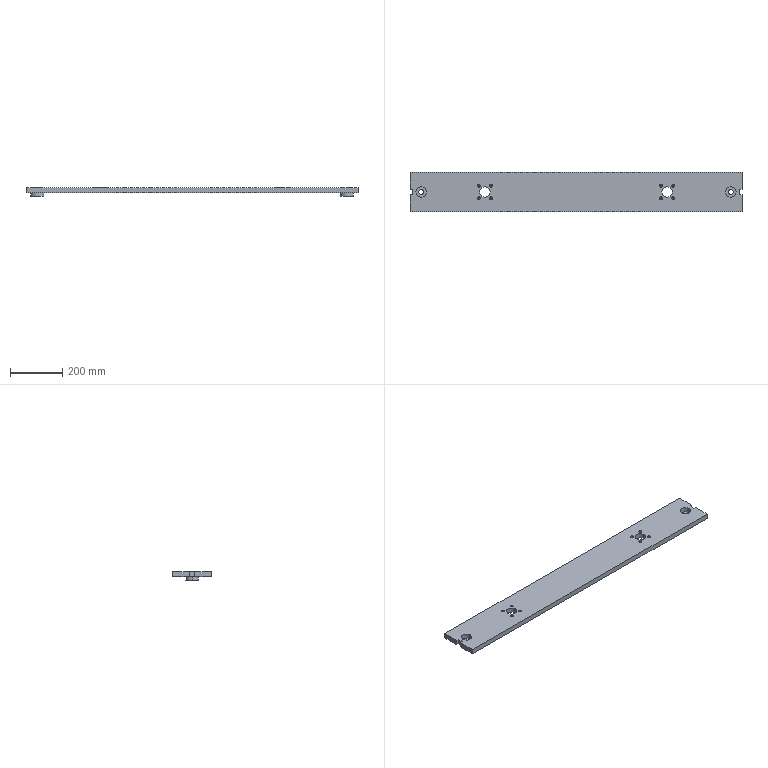Part | SolidWorks | features ICE 3, Cut 1, Extrusion 1 | 3 solids | 74 faces | box 1276 x 150 x 34 mm | volume 3757893 mm3 | cylinder 48 | plane 26 | commonest cylinder face diameters 7 x16 11 x16 40 x8 18 x4 50 x4